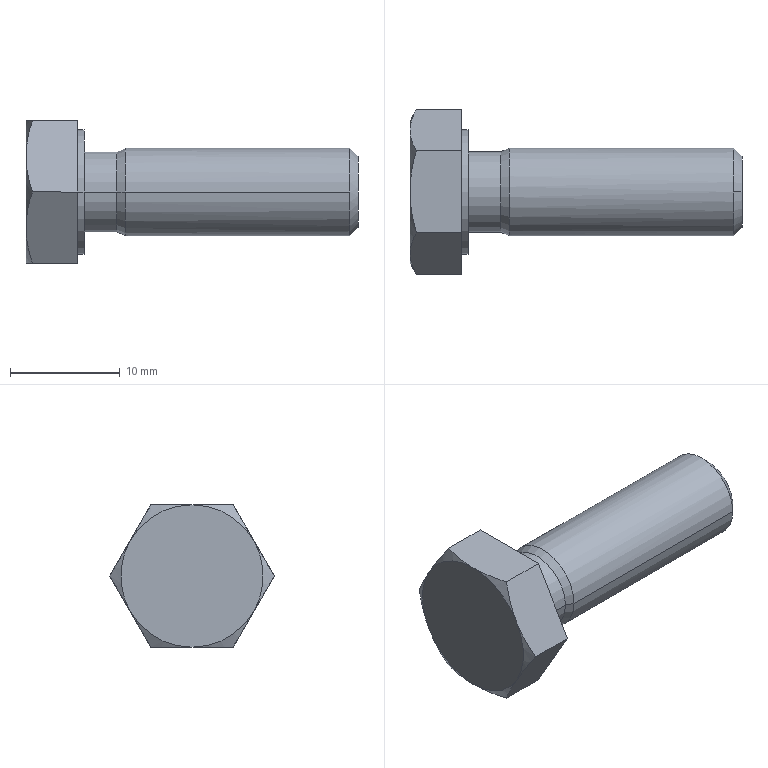Part | SolidWorks | features BaseBody 1 | 1 solid | 26 faces | box 30.3 x 15.011 x 13 mm | volume 1969 mm3 | cone 10 | plane 10 | cylinder 6 | commonest cylinder face diameters 7.323 x2 8 x2 11.4 x2
STEP:
#1=CARTESIAN_POINT('',(3.75,4.,0.));
#2=VERTEX_POINT('',#1);
#3=CARTESIAN_POINT('',(3.75,-4.,0.));
#4=VERTEX_POINT('',#3);
#5=CARTESIAN_POINT('',(3.75,0.,0.));
#6=DIRECTION('',(1.,0.,0.));
#7=DIRECTION('',(0.,1.,0.));
#8=AXIS2_PLACEMENT_3D('',#5,#6,#7);
#9=CIRCLE('',#8,4.);
#10=EDGE_CURVE('',#2,#4,#9,.T.);
#11=ORIENTED_EDGE('',*,*,#10,.T.);
#12=CARTESIAN_POINT('',(24.233,-4.,0.));
#13=VERTEX_POINT('',#12);
#14=CARTESIAN_POINT('',(14.375,-4.,0.));
#15=DIRECTION('',(1.,0.,0.));
#16=VECTOR('',#15,1000.);
#17=LINE('',#14,#16);
#18=EDGE_CURVE('',#4,#13,#17,.T.);
#19=ORIENTED_EDGE('',*,*,#18,.T.);
#20=CARTESIAN_POINT('',(24.233,0.,4.));
#21=VERTEX_POINT('',#20);
#22=CARTESIAN_POINT('',(24.233,0.,0.));
#23=DIRECTION('',(-1.,0.,0.));
#24=DIRECTION('',(0.,1.,0.));
#25=AXIS2_PLACEMENT_3D('',#22,#23,#24);
#26=CIRCLE('',#25,4.);
#27=EDGE_CURVE('',#13,#21,#26,.T.);
#28=ORIENTED_EDGE('',*,*,#27,.T.);
#29=CARTESIAN_POINT('',(24.233,4.,0.));
#30=VERTEX_POINT('',#29);
#31=CARTESIAN_POINT('',(24.233,0.,0.));
#32=DIRECTION('',(-1.,0.,0.));
#33=DIRECTION('',(0.,1.,0.));
#34=AXIS2_PLACEMENT_3D('',#31,#32,#33);
#35=CIRCLE('',#34,4.);
#36=EDGE_CURVE('',#21,#30,#35,.T.);
#37=ORIENTED_EDGE('',*,*,#36,.T.);
#38=CARTESIAN_POINT('',(14.375,4.,0.));
#39=DIRECTION('',(1.,0.,0.));
#40=VECTOR('',#39,1000.);
#41=LINE('',#38,#40);
#42=EDGE_CURVE('',#2,#30,#41,.T.);
#43=ORIENTED_EDGE('',*,*,#42,.F.);
#44=EDGE_LOOP('',(#11,#19,#28,#37,#43));
#45=FACE_OUTER_BOUND('',#44,.T.);
#46=CARTESIAN_POINT('',(14.375,0.,0.));
#47=DIRECTION('',(1.,0.,0.));
#48=DIRECTION('',(0.,1.,0.));
#49=AXIS2_PLACEMENT_3D('',#46,#47,#48);
#50=CYLINDRICAL_SURFACE('',#49,4.);
#51=ADVANCED_FACE('',(#45),#50,.T.);
#52=CARTESIAN_POINT('',(25.,0.,3.233));
#53=VERTEX_POINT('',#52);
#54=CARTESIAN_POINT('',(25.,0.,-3.233));
#55=VERTEX_POINT('',#54);
#56=CARTESIAN_POINT('',(25.,0.,0.));
#57=DIRECTION('',(-1.,0.,0.));
#58=DIRECTION('',(0.,0.,1.));
#59=AXIS2_PLACEMENT_3D('',#56,#57,#58);
#60=CIRCLE('',#59,3.233);
#61=EDGE_CURVE('',#53,#55,#60,.T.);
#62=ORIENTED_EDGE('',*,*,#61,.T.);
#63=CARTESIAN_POINT('',(24.233,0.,-4.));
#64=VERTEX_POINT('',#63);
#65=CARTESIAN_POINT('',(24.233,0.,-4.));
#66=DIRECTION('',(-0.7072,0.,-0.7071));
#67=VECTOR('',#66,1000.);
#68=LINE('',#65,#67);
#69=EDGE_CURVE('',#55,#64,#68,.T.);
#70=ORIENTED_EDGE('',*,*,#69,.T.);
#71=CARTESIAN_POINT('',(24.233,0.,0.));
#72=DIRECTION('',(-1.,0.,0.));
#73=DIRECTION('',(0.,1.,0.));
#74=AXIS2_PLACEMENT_3D('',#71,#72,#73);
#75=CIRCLE('',#74,4.);
#76=EDGE_CURVE('',#30,#64,#75,.T.);
#77=ORIENTED_EDGE('',*,*,#76,.F.);
#78=ORIENTED_EDGE('',*,*,#36,.F.);
#79=CARTESIAN_POINT('',(24.233,0.,4.));
#80=DIRECTION('',(-0.7072,0.,0.7071));
#81=VECTOR('',#80,1000.);
#82=LINE('',#79,#81);
#83=EDGE_CURVE('',#53,#21,#82,.T.);
#84=ORIENTED_EDGE('',*,*,#83,.F.);
#85=EDGE_LOOP('',(#62,#70,#77,#78,#84));
#86=FACE_OUTER_BOUND('',#85,.T.);
#87=CARTESIAN_POINT('',(24.233,0.,0.));
#88=DIRECTION('',(-1.,0.,0.));
#89=DIRECTION('',(0.,0.,1.));
#90=AXIS2_PLACEMENT_3D('',#87,#88,#89);
#91=CONICAL_SURFACE('',#90,4.,0.7853);
#92=ADVANCED_FACE('',(#86),#91,.T.);
#93=CARTESIAN_POINT('',(2.983,3.662,0.));
#94=VERTEX_POINT('',#93);
#95=CARTESIAN_POINT('',(2.983,-3.662,0.));
#96=VERTEX_POINT('',#95);
#97=CARTESIAN_POINT('',(2.983,0.,0.));
#98=DIRECTION('',(1.,0.,0.));
#99=DIRECTION('',(0.,1.,0.));
#100=AXIS2_PLACEMENT_3D('',#97,#98,#99);
#101=CIRCLE('',#100,3.662);
#102=EDGE_CURVE('',#94,#96,#101,.T.);
#103=ORIENTED_EDGE('',*,*,#102,.T.);
#104=CARTESIAN_POINT('',(3.75,-4.,0.));
#105=DIRECTION('',(0.9149,-0.4036,0.));
#106=VECTOR('',#105,1000.);
#107=LINE('',#104,#106);
#108=EDGE_CURVE('',#96,#4,#107,.T.);
#109=ORIENTED_EDGE('',*,*,#108,.T.);
#110=ORIENTED_EDGE('',*,*,#10,.F.);
#111=CARTESIAN_POINT('',(3.75,4.,0.));
#112=DIRECTION('',(0.9149,0.4036,0.));
#113=VECTOR('',#112,1000.);
#114=LINE('',#111,#113);
#115=EDGE_CURVE('',#94,#2,#114,.T.);
#116=ORIENTED_EDGE('',*,*,#115,.F.);
#117=EDGE_LOOP('',(#103,#109,#110,#116));
#118=FACE_OUTER_BOUND('',#117,.T.);
#119=CARTESIAN_POINT('',(3.75,0.,0.));
#120=DIRECTION('',(1.,0.,0.));
#121=DIRECTION('',(0.,1.,0.));
#122=AXIS2_PLACEMENT_3D('',#119,#120,#121);
#123=CONICAL_SURFACE('',#122,4.,0.4154);
#124=ADVANCED_FACE('',(#118),#123,.T.);
#125=CARTESIAN_POINT('',(0.,3.662,0.));
#126=VERTEX_POINT('',#125);
#127=CARTESIAN_POINT('',(0.,-3.662,0.));
#128=VERTEX_POINT('',#127);
#129=CARTESIAN_POINT('',(0.,0.,0.));
#130=DIRECTION('',(1.,0.,0.));
#131=DIRECTION('',(0.,1.,0.));
#132=AXIS2_PLACEMENT_3D('',#129,#130,#131);
#133=CIRCLE('',#132,3.662);
#134=EDGE_CURVE('',#126,#128,#133,.T.);
#135=ORIENTED_EDGE('',*,*,#134,.T.);
#136=CARTESIAN_POINT('',(1.492,-3.662,0.));
#137=DIRECTION('',(1.,0.,0.));
#138=VECTOR('',#137,1000.);
#139=LINE('',#136,#138);
#140=EDGE_CURVE('',#128,#96,#139,.T.);
#141=ORIENTED_EDGE('',*,*,#140,.T.);
#142=ORIENTED_EDGE('',*,*,#102,.F.);
#143=CARTESIAN_POINT('',(1.492,3.662,0.));
#144=DIRECTION('',(1.,0.,0.));
#145=VECTOR('',#144,1000.);
#146=LINE('',#143,#145);
#147=EDGE_CURVE('',#126,#94,#146,.T.);
#148=ORIENTED_EDGE('',*,*,#147,.F.);
#149=EDGE_LOOP('',(#135,#141,#142,#148));
#150=FACE_OUTER_BOUND('',#149,.T.);
#151=CARTESIAN_POINT('',(1.492,0.,0.));
#152=DIRECTION('',(1.,0.,0.));
#153=DIRECTION('',(0.,1.,0.));
#154=AXIS2_PLACEMENT_3D('',#151,#152,#153);
#155=CYLINDRICAL_SURFACE('',#154,3.662);
#156=ADVANCED_FACE('',(#150),#155,.T.);
#157=CARTESIAN_POINT('',(-0.6001,5.7,0.));
#158=VERTEX_POINT('',#157);
#159=CARTESIAN_POINT('',(-0.6001,-5.7,0.));
#160=VERTEX_POINT('',#159);
#161=CARTESIAN_POINT('',(-0.6001,0.,0.));
#162=DIRECTION('',(1.,0.,0.));
#163=DIRECTION('',(0.,1.,0.));
#164=AXIS2_PLACEMENT_3D('',#161,#162,#163);
#165=CIRCLE('',#164,5.7);
#166=EDGE_CURVE('',#158,#160,#165,.T.);
#167=ORIENTED_EDGE('',*,*,#166,.T.);
#168=CARTESIAN_POINT('',(0.,-5.7,0.));
#169=VERTEX_POINT('',#168);
#170=CARTESIAN_POINT('',(-0.3,-5.7,0.));
#171=DIRECTION('',(1.,0.,0.));
#172=VECTOR('',#171,1000.);
#173=LINE('',#170,#172);
#174=EDGE_CURVE('',#160,#169,#173,.T.);
#175=ORIENTED_EDGE('',*,*,#174,.T.);
#176=CARTESIAN_POINT('',(0.,5.7,0.));
#177=VERTEX_POINT('',#176);
#178=CARTESIAN_POINT('',(0.,0.,0.));
#179=DIRECTION('',(1.,0.,0.));
#180=DIRECTION('',(0.,1.,0.));
#181=AXIS2_PLACEMENT_3D('',#178,#179,#180);
#182=CIRCLE('',#181,5.7);
#183=EDGE_CURVE('',#177,#169,#182,.T.);
#184=ORIENTED_EDGE('',*,*,#183,.F.);
#185=CARTESIAN_POINT('',(-0.3,5.7,0.));
#186=DIRECTION('',(1.,0.,0.));
#187=VECTOR('',#186,1000.);
#188=LINE('',#185,#187);
#189=EDGE_CURVE('',#158,#177,#188,.T.);
#190=ORIENTED_EDGE('',*,*,#189,.F.);
#191=EDGE_LOOP('',(#167,#175,#184,#190));
#192=FACE_OUTER_BOUND('',#191,.T.);
#193=CARTESIAN_POINT('',(-0.3,0.,0.));
#194=DIRECTION('',(1.,0.,0.));
#195=DIRECTION('',(0.,1.,0.));
#196=AXIS2_PLACEMENT_3D('',#193,#194,#195);
#197=CYLINDRICAL_SURFACE('',#196,5.7);
#198=ADVANCED_FACE('',(#192),#197,.T.);
#199=ORIENTED_EDGE('',*,*,#18,.F.);
#200=CARTESIAN_POINT('',(3.75,0.,0.));
#201=DIRECTION('',(1.,0.,0.));
#202=DIRECTION('',(0.,1.,0.));
#203=AXIS2_PLACEMENT_3D('',#200,#201,#202);
#204=CIRCLE('',#203,4.);
#205=EDGE_CURVE('',#4,#2,#204,.T.);
#206=ORIENTED_EDGE('',*,*,#205,.T.);
#207=ORIENTED_EDGE('',*,*,#42,.T.);
#208=ORIENTED_EDGE('',*,*,#76,.T.);
#209=CARTESIAN_POINT('',(24.233,0.,0.));
#210=DIRECTION('',(-1.,0.,0.));
#211=DIRECTION('',(0.,1.,0.));
#212=AXIS2_PLACEMENT_3D('',#209,#210,#211);
#213=CIRCLE('',#212,4.);
#214=EDGE_CURVE('',#64,#13,#213,.T.);
#215=ORIENTED_EDGE('',*,*,#214,.T.);
#216=EDGE_LOOP('',(#199,#206,#207,#208,#215));
#217=FACE_OUTER_BOUND('',#216,.T.);
#218=CARTESIAN_POINT('',(14.375,0.,0.));
#219=DIRECTION('',(1.,0.,0.));
#220=DIRECTION('',(0.,1.,0.));
#221=AXIS2_PLACEMENT_3D('',#218,#219,#220);
#222=CYLINDRICAL_SURFACE('',#221,4.);
#223=ADVANCED_FACE('',(#217),#222,.T.);
#224=ORIENTED_EDGE('',*,*,#69,.F.);
#225=CARTESIAN_POINT('',(25.,0.,0.));
#226=DIRECTION('',(-1.,0.,0.));
#227=DIRECTION('',(0.,0.,1.));
#228=AXIS2_PLACEMENT_3D('',#225,#226,#227);
#229=CIRCLE('',#228,3.233);
#230=EDGE_CURVE('',#55,#53,#229,.T.);
#231=ORIENTED_EDGE('',*,*,#230,.T.);
#232=ORIENTED_EDGE('',*,*,#83,.T.);
#233=ORIENTED_EDGE('',*,*,#27,.F.);
#234=ORIENTED_EDGE('',*,*,#214,.F.);
#235=EDGE_LOOP('',(#224,#231,#232,#233,#234));
#236=FACE_OUTER_BOUND('',#235,.T.);
#237=CARTESIAN_POINT('',(24.233,0.,0.));
#238=DIRECTION('',(-1.,0.,0.));
#239=DIRECTION('',(0.,0.,1.));
#240=AXIS2_PLACEMENT_3D('',#237,#238,#239);
#241=CONICAL_SURFACE('',#240,4.,0.7853);
#242=ADVANCED_FACE('',(#236),#241,.T.);
#243=ORIENTED_EDGE('',*,*,#108,.F.);
#244=CARTESIAN_POINT('',(2.983,0.,0.));
#245=DIRECTION('',(1.,0.,0.));
#246=DIRECTION('',(0.,1.,0.));
#247=AXIS2_PLACEMENT_3D('',#244,#245,#246);
#248=CIRCLE('',#247,3.662);
#249=EDGE_CURVE('',#96,#94,#248,.T.);
#250=ORIENTED_EDGE('',*,*,#249,.T.);
#251=ORIENTED_EDGE('',*,*,#115,.T.);
#252=ORIENTED_EDGE('',*,*,#205,.F.);
#253=EDGE_LOOP('',(#243,#250,#251,#252));
#254=FACE_OUTER_BOUND('',#253,.T.);
#255=CARTESIAN_POINT('',(3.75,0.,0.));
#256=DIRECTION('',(1.,0.,0.));
#257=DIRECTION('',(0.,1.,0.));
#258=AXIS2_PLACEMENT_3D('',#255,#256,#257);
#259=CONICAL_SURFACE('',#258,4.,0.4154);
#260=ADVANCED_FACE('',(#254),#259,.T.);
#261=ORIENTED_EDGE('',*,*,#61,.F.);
#262=ORIENTED_EDGE('',*,*,#230,.F.);
#263=EDGE_LOOP('',(#261,#262));
#264=FACE_OUTER_BOUND('',#263,.T.);
#265=CARTESIAN_POINT('',(25.,2.,0.));
#266=DIRECTION('',(1.,0.,0.));
#267=DIRECTION('',(0.,1.,0.));
#268=AXIS2_PLACEMENT_3D('',#265,#266,#267);
#269=PLANE('',#268);
#270=ADVANCED_FACE('',(#264),#269,.T.);
#271=ORIENTED_EDGE('',*,*,#140,.F.);
#272=CARTESIAN_POINT('',(0.,0.,0.));
#273=DIRECTION('',(1.,0.,0.));
#274=DIRECTION('',(0.,1.,0.));
#275=AXIS2_PLACEMENT_3D('',#272,#273,#274);
#276=CIRCLE('',#275,3.662);
#277=EDGE_CURVE('',#128,#126,#276,.T.);
#278=ORIENTED_EDGE('',*,*,#277,.T.);
#279=ORIENTED_EDGE('',*,*,#147,.T.);
#280=ORIENTED_EDGE('',*,*,#249,.F.);
#281=EDGE_LOOP('',(#271,#278,#279,#280));
#282=FACE_OUTER_BOUND('',#281,.T.);
#283=CARTESIAN_POINT('',(1.492,0.,0.));
#284=DIRECTION('',(1.,0.,0.));
#285=DIRECTION('',(0.,1.,0.));
#286=AXIS2_PLACEMENT_3D('',#283,#284,#285);
#287=CYLINDRICAL_SURFACE('',#286,3.662);
#288=ADVANCED_FACE('',(#282),#287,.T.);
#289=ORIENTED_EDGE('',*,*,#134,.F.);
#290=ORIENTED_EDGE('',*,*,#277,.F.);
#291=EDGE_LOOP('',(#289,#290));
#292=FACE_BOUND('',#291,.T.);
#293=ORIENTED_EDGE('',*,*,#183,.T.);
#294=CARTESIAN_POINT('',(0.,0.,0.));
#295=DIRECTION('',(1.,0.,0.));
#296=DIRECTION('',(0.,1.,0.));
#297=AXIS2_PLACEMENT_3D('',#294,#295,#296);
#298=CIRCLE('',#297,5.7);
#299=EDGE_CURVE('',#169,#177,#298,.T.);
#300=ORIENTED_EDGE('',*,*,#299,.T.);
#301=EDGE_LOOP('',(#293,#300));
#302=FACE_OUTER_BOUND('',#301,.T.);
#303=CARTESIAN_POINT('',(0.,4.681,0.));
#304=DIRECTION('',(1.,0.,0.));
#305=DIRECTION('',(0.,1.,0.));
#306=AXIS2_PLACEMENT_3D('',#303,#304,#305);
#307=PLANE('',#306);
#308=ADVANCED_FACE('',(#292,#302),#307,.T.);
#309=ORIENTED_EDGE('',*,*,#174,.F.);
#310=CARTESIAN_POINT('',(-0.6001,0.,0.));
#311=DIRECTION('',(1.,0.,0.));
#312=DIRECTION('',(0.,1.,0.));
#313=AXIS2_PLACEMENT_3D('',#310,#311,#312);
#314=CIRCLE('',#313,5.7);
#315=EDGE_CURVE('',#160,#158,#314,.T.);
#316=ORIENTED_EDGE('',*,*,#315,.T.);
#317=ORIENTED_EDGE('',*,*,#189,.T.);
#318=ORIENTED_EDGE('',*,*,#299,.F.);
#319=EDGE_LOOP('',(#309,#316,#317,#318));
#320=FACE_OUTER_BOUND('',#319,.T.);
#321=CARTESIAN_POINT('',(-0.3,0.,0.));
#322=DIRECTION('',(1.,0.,0.));
#323=DIRECTION('',(0.,1.,0.));
#324=AXIS2_PLACEMENT_3D('',#321,#322,#323);
#325=CYLINDRICAL_SURFACE('',#324,5.7);
#326=ADVANCED_FACE('',(#320),#325,.T.);
#327=ORIENTED_EDGE('',*,*,#166,.F.);
#328=ORIENTED_EDGE('',*,*,#315,.F.);
#329=EDGE_LOOP('',(#327,#328));
#330=FACE_BOUND('',#329,.T.);
#331=CARTESIAN_POINT('',(-0.6001,-3.753,-6.5));
#332=VERTEX_POINT('',#331);
#333=CARTESIAN_POINT('',(-0.6001,3.753,-6.5));
#334=VERTEX_POINT('',#333);
#335=CARTESIAN_POINT('',(-0.6001,0.,-6.5));
#336=DIRECTION('',(0.,1.,0.));
#337=VECTOR('',#336,1000.);
#338=LINE('',#335,#337);
#339=EDGE_CURVE('',#332,#334,#338,.T.);
#340=ORIENTED_EDGE('',*,*,#339,.T.);
#341=CARTESIAN_POINT('',(-0.6001,7.506,0.));
#342=VERTEX_POINT('',#341);
#343=CARTESIAN_POINT('',(-0.6001,3.753,-6.5));
#344=DIRECTION('',(0.,0.5,0.866));
#345=VECTOR('',#344,1000.);
#346=LINE('',#343,#345);
#347=EDGE_CURVE('',#334,#342,#346,.T.);
#348=ORIENTED_EDGE('',*,*,#347,.T.);
#349=CARTESIAN_POINT('',(-0.6001,3.753,6.5));
#350=VERTEX_POINT('',#349);
#351=CARTESIAN_POINT('',(-0.6001,7.506,0.));
#352=DIRECTION('',(0.,-0.5,0.866));
#353=VECTOR('',#352,1000.);
#354=LINE('',#351,#353);
#355=EDGE_CURVE('',#342,#350,#354,.T.);
#356=ORIENTED_EDGE('',*,*,#355,.T.);
#357=CARTESIAN_POINT('',(-0.6001,-3.753,6.5));
#358=VERTEX_POINT('',#357);
#359=CARTESIAN_POINT('',(-0.6001,0.,6.5));
#360=DIRECTION('',(0.,-1.,0.));
#361=VECTOR('',#360,1000.);
#362=LINE('',#359,#361);
#363=EDGE_CURVE('',#350,#358,#362,.T.);
#364=ORIENTED_EDGE('',*,*,#363,.T.);
#365=CARTESIAN_POINT('',(-0.6001,-7.506,0.));
#366=VERTEX_POINT('',#365);
#367=CARTESIAN_POINT('',(-0.6001,-3.753,6.5));
#368=DIRECTION('',(0.,-0.5,-0.866));
#369=VECTOR('',#368,1000.);
#370=LINE('',#367,#369);
#371=EDGE_CURVE('',#358,#366,#370,.T.);
#372=ORIENTED_EDGE('',*,*,#371,.T.);
#373=CARTESIAN_POINT('',(-0.6001,-7.506,0.));
#374=DIRECTION('',(0.,0.5,-0.866));
#375=VECTOR('',#374,1000.);
#376=LINE('',#373,#375);
#377=EDGE_CURVE('',#366,#332,#376,.T.);
#378=ORIENTED_EDGE('',*,*,#377,.T.);
#379=EDGE_LOOP('',(#340,#348,#356,#364,#372,#378));
#380=FACE_OUTER_BOUND('',#379,.T.);
#381=CARTESIAN_POINT('',(-0.6001,0.,0.));
#382=DIRECTION('',(1.,0.,0.));
#383=DIRECTION('',(0.,1.,0.));
#384=AXIS2_PLACEMENT_3D('',#381,#382,#383);
#385=PLANE('',#384);
#386=ADVANCED_FACE('',(#330,#380),#385,.T.);
#387=ORIENTED_EDGE('',*,*,#347,.F.);
#388=CARTESIAN_POINT('',(-4.72,3.753,-6.5));
#389=VERTEX_POINT('',#388);
#390=CARTESIAN_POINT('',(-0.6001,3.753,-6.5));
#391=DIRECTION('',(-1.,0.,0.));
#392=VECTOR('',#391,1000.);
#393=LINE('',#390,#392);
#394=EDGE_CURVE('',#334,#389,#393,.T.);
#395=ORIENTED_EDGE('',*,*,#394,.T.);
#396=CARTESIAN_POINT('',(-5.3,5.629,-3.25));
#397=VERTEX_POINT('',#396);
#398=CARTESIAN_POINT('',(-4.72,3.753,-6.5));
#399=CARTESIAN_POINT('',(-5.073,4.366,-5.438));
#400=CARTESIAN_POINT('',(-5.3,4.989,-4.359));
#401=CARTESIAN_POINT('',(-5.3,5.629,-3.25));
#402=B_SPLINE_CURVE_WITH_KNOTS('',3,(#398,#399,#400,#401),.UNSPECIFIED.,.F.,.F.,(4,4),(0.,0.003797),.UNSPECIFIED.);
#403=EDGE_CURVE('',#389,#397,#402,.T.);
#404=ORIENTED_EDGE('',*,*,#403,.T.);
#405=CARTESIAN_POINT('',(-4.72,7.506,0.));
#406=VERTEX_POINT('',#405);
#407=CARTESIAN_POINT('',(-5.3,5.629,-3.25));
#408=CARTESIAN_POINT('',(-5.3,6.27,-2.141));
#409=CARTESIAN_POINT('',(-5.073,6.892,-1.062));
#410=CARTESIAN_POINT('',(-4.72,7.506,0.));
#411=B_SPLINE_CURVE_WITH_KNOTS('',3,(#407,#408,#409,#410),.UNSPECIFIED.,.F.,.F.,(4,4),(0.,0.003797),.UNSPECIFIED.);
#412=EDGE_CURVE('',#397,#406,#411,.T.);
#413=ORIENTED_EDGE('',*,*,#412,.T.);
#414=CARTESIAN_POINT('',(-0.6001,7.506,0.));
#415=DIRECTION('',(1.,0.,0.));
#416=VECTOR('',#415,1000.);
#417=LINE('',#414,#416);
#418=EDGE_CURVE('',#406,#342,#417,.T.);
#419=ORIENTED_EDGE('',*,*,#418,.T.);
#420=EDGE_LOOP('',(#387,#395,#404,#413,#419));
#421=FACE_OUTER_BOUND('',#420,.T.);
#422=CARTESIAN_POINT('',(-0.6001,3.753,-6.5));
#423=DIRECTION('',(0.,0.866,-0.5));
#424=DIRECTION('',(0.,0.5,0.866));
#425=AXIS2_PLACEMENT_3D('',#422,#423,#424);
#426=PLANE('',#425);
#427=ADVANCED_FACE('',(#421),#426,.T.);
#428=ORIENTED_EDGE('',*,*,#339,.F.);
#429=CARTESIAN_POINT('',(-4.72,-3.753,-6.5));
#430=VERTEX_POINT('',#429);
#431=CARTESIAN_POINT('',(-0.6001,-3.753,-6.5));
#432=DIRECTION('',(-1.,0.,0.));
#433=VECTOR('',#432,1000.);
#434=LINE('',#431,#433);
#435=EDGE_CURVE('',#332,#430,#434,.T.);
#436=ORIENTED_EDGE('',*,*,#435,.T.);
#437=CARTESIAN_POINT('',(-5.3,0.,-6.5));
#438=VERTEX_POINT('',#437);
#439=CARTESIAN_POINT('',(-4.72,-3.753,-6.5));
#440=CARTESIAN_POINT('',(-5.073,-2.527,-6.5));
#441=CARTESIAN_POINT('',(-5.3,-1.281,-6.5));
#442=CARTESIAN_POINT('',(-5.3,0.,-6.5));
#443=B_SPLINE_CURVE_WITH_KNOTS('',3,(#439,#440,#441,#442),.UNSPECIFIED.,.F.,.F.,(4,4),(0.,0.003797),.UNSPECIFIED.);
#444=EDGE_CURVE('',#430,#438,#443,.T.);
#445=ORIENTED_EDGE('',*,*,#444,.T.);
#446=CARTESIAN_POINT('',(-5.3,0.,-6.5));
#447=CARTESIAN_POINT('',(-5.3,1.281,-6.5));
#448=CARTESIAN_POINT('',(-5.073,2.527,-6.5));
#449=CARTESIAN_POINT('',(-4.72,3.753,-6.5));
#450=B_SPLINE_CURVE_WITH_KNOTS('',3,(#446,#447,#448,#449),.UNSPECIFIED.,.F.,.F.,(4,4),(0.,0.003797),.UNSPECIFIED.);
#451=EDGE_CURVE('',#438,#389,#450,.T.);
#452=ORIENTED_EDGE('',*,*,#451,.T.);
#453=ORIENTED_EDGE('',*,*,#394,.F.);
#454=EDGE_LOOP('',(#428,#436,#445,#452,#453));
#455=FACE_OUTER_BOUND('',#454,.T.);
#456=CARTESIAN_POINT('',(-0.6001,-3.753,-6.5));
#457=DIRECTION('',(0.,0.,-1.));
#458=DIRECTION('',(0.,1.,0.));
#459=AXIS2_PLACEMENT_3D('',#456,#457,#458);
#460=PLANE('',#459);
#461=ADVANCED_FACE('',(#455),#460,.T.);
#462=CARTESIAN_POINT('',(-4.72,-7.506,0.));
#463=VERTEX_POINT('',#462);
#464=CARTESIAN_POINT('',(-0.6001,-7.506,0.));
#465=DIRECTION('',(-1.,0.,0.));
#466=VECTOR('',#465,1000.);
#467=LINE('',#464,#466);
#468=EDGE_CURVE('',#366,#463,#467,.T.);
#469=ORIENTED_EDGE('',*,*,#468,.T.);
#470=CARTESIAN_POINT('',(-5.3,-5.629,-3.25));
#471=VERTEX_POINT('',#470);
#472=CARTESIAN_POINT('',(-4.72,-7.506,0.));
#473=CARTESIAN_POINT('',(-5.073,-6.892,-1.062));
#474=CARTESIAN_POINT('',(-5.3,-6.27,-2.141));
#475=CARTESIAN_POINT('',(-5.3,-5.629,-3.25));
#476=B_SPLINE_CURVE_WITH_KNOTS('',3,(#472,#473,#474,#475),.UNSPECIFIED.,.F.,.F.,(4,4),(0.,0.003797),.UNSPECIFIED.);
#477=EDGE_CURVE('',#463,#471,#476,.T.);
#478=ORIENTED_EDGE('',*,*,#477,.T.);
#479=CARTESIAN_POINT('',(-5.3,-5.629,-3.25));
#480=CARTESIAN_POINT('',(-5.3,-4.989,-4.359));
#481=CARTESIAN_POINT('',(-5.073,-4.366,-5.438));
#482=CARTESIAN_POINT('',(-4.72,-3.753,-6.5));
#483=B_SPLINE_CURVE_WITH_KNOTS('',3,(#479,#480,#481,#482),.UNSPECIFIED.,.F.,.F.,(4,4),(0.,0.003797),.UNSPECIFIED.);
#484=EDGE_CURVE('',#471,#430,#483,.T.);
#485=ORIENTED_EDGE('',*,*,#484,.T.);
#486=ORIENTED_EDGE('',*,*,#435,.F.);
#487=ORIENTED_EDGE('',*,*,#377,.F.);
#488=EDGE_LOOP('',(#469,#478,#485,#486,#487));
#489=FACE_OUTER_BOUND('',#488,.T.);
#490=CARTESIAN_POINT('',(-0.6001,-7.506,0.));
#491=DIRECTION('',(0.,-0.866,-0.5));
#492=DIRECTION('',(0.,0.5,-0.866));
#493=AXIS2_PLACEMENT_3D('',#490,#491,#492);
#494=PLANE('',#493);
#495=ADVANCED_FACE('',(#489),#494,.T.);
#496=CARTESIAN_POINT('',(-4.72,-3.753,6.5));
#497=VERTEX_POINT('',#496);
#498=CARTESIAN_POINT('',(-0.6001,-3.753,6.5));
#499=DIRECTION('',(-1.,0.,0.));
#500=VECTOR('',#499,1000.);
#501=LINE('',#498,#500);
#502=EDGE_CURVE('',#358,#497,#501,.T.);
#503=ORIENTED_EDGE('',*,*,#502,.T.);
#504=CARTESIAN_POINT('',(-5.3,-5.629,3.25));
#505=VERTEX_POINT('',#504);
#506=CARTESIAN_POINT('',(-4.72,-3.753,6.5));
#507=CARTESIAN_POINT('',(-5.073,-4.366,5.438));
#508=CARTESIAN_POINT('',(-5.3,-4.989,4.359));
#509=CARTESIAN_POINT('',(-5.3,-5.629,3.25));
#510=B_SPLINE_CURVE_WITH_KNOTS('',3,(#506,#507,#508,#509),.UNSPECIFIED.,.F.,.F.,(4,4),(0.,0.003797),.UNSPECIFIED.);
#511=EDGE_CURVE('',#497,#505,#510,.T.);
#512=ORIENTED_EDGE('',*,*,#511,.T.);
#513=CARTESIAN_POINT('',(-5.3,-5.629,3.25));
#514=CARTESIAN_POINT('',(-5.3,-6.27,2.141));
#515=CARTESIAN_POINT('',(-5.073,-6.892,1.062));
#516=CARTESIAN_POINT('',(-4.72,-7.506,0.));
#517=B_SPLINE_CURVE_WITH_KNOTS('',3,(#513,#514,#515,#516),.UNSPECIFIED.,.F.,.F.,(4,4),(0.,0.003797),.UNSPECIFIED.);
#518=EDGE_CURVE('',#505,#463,#517,.T.);
#519=ORIENTED_EDGE('',*,*,#518,.T.);
#520=ORIENTED_EDGE('',*,*,#468,.F.);
#521=ORIENTED_EDGE('',*,*,#371,.F.);
#522=EDGE_LOOP('',(#503,#512,#519,#520,#521));
#523=FACE_OUTER_BOUND('',#522,.T.);
#524=CARTESIAN_POINT('',(-0.6001,-3.753,6.5));
#525=DIRECTION('',(0.,-0.866,0.5));
#526=DIRECTION('',(0.,-0.5,-0.866));
#527=AXIS2_PLACEMENT_3D('',#524,#525,#526);
#528=PLANE('',#527);
#529=ADVANCED_FACE('',(#523),#528,.T.);
#530=CARTESIAN_POINT('',(-4.72,3.753,6.5));
#531=VERTEX_POINT('',#530);
#532=CARTESIAN_POINT('',(-0.6001,3.753,6.5));
#533=DIRECTION('',(-1.,0.,0.));
#534=VECTOR('',#533,1000.);
#535=LINE('',#532,#534);
#536=EDGE_CURVE('',#350,#531,#535,.T.);
#537=ORIENTED_EDGE('',*,*,#536,.T.);
#538=CARTESIAN_POINT('',(-5.3,0.,6.5));
#539=VERTEX_POINT('',#538);
#540=CARTESIAN_POINT('',(-4.72,3.753,6.5));
#541=CARTESIAN_POINT('',(-5.073,2.527,6.5));
#542=CARTESIAN_POINT('',(-5.3,1.281,6.5));
#543=CARTESIAN_POINT('',(-5.3,0.,6.5));
#544=B_SPLINE_CURVE_WITH_KNOTS('',3,(#540,#541,#542,#543),.UNSPECIFIED.,.F.,.F.,(4,4),(0.,0.003797),.UNSPECIFIED.);
#545=EDGE_CURVE('',#531,#539,#544,.T.);
#546=ORIENTED_EDGE('',*,*,#545,.T.);
#547=CARTESIAN_POINT('',(-5.3,0.,6.5));
#548=CARTESIAN_POINT('',(-5.3,-1.281,6.5));
#549=CARTESIAN_POINT('',(-5.073,-2.527,6.5));
#550=CARTESIAN_POINT('',(-4.72,-3.753,6.5));
#551=B_SPLINE_CURVE_WITH_KNOTS('',3,(#547,#548,#549,#550),.UNSPECIFIED.,.F.,.F.,(4,4),(0.,0.003797),.UNSPECIFIED.);
#552=EDGE_CURVE('',#539,#497,#551,.T.);
#553=ORIENTED_EDGE('',*,*,#552,.T.);
#554=ORIENTED_EDGE('',*,*,#502,.F.);
#555=ORIENTED_EDGE('',*,*,#363,.F.);
#556=EDGE_LOOP('',(#537,#546,#553,#554,#555));
#557=FACE_OUTER_BOUND('',#556,.T.);
#558=CARTESIAN_POINT('',(-0.6001,3.753,6.5));
#559=DIRECTION('',(0.,0.,1.));
#560=DIRECTION('',(0.,-1.,0.));
#561=AXIS2_PLACEMENT_3D('',#558,#559,#560);
#562=PLANE('',#561);
#563=ADVANCED_FACE('',(#557),#562,.T.);
#564=ORIENTED_EDGE('',*,*,#355,.F.);
#565=ORIENTED_EDGE('',*,*,#418,.F.);
#566=CARTESIAN_POINT('',(-5.3,5.629,3.25));
#567=VERTEX_POINT('',#566);
#568=CARTESIAN_POINT('',(-4.72,7.506,0.));
#569=CARTESIAN_POINT('',(-5.073,6.892,1.062));
#570=CARTESIAN_POINT('',(-5.3,6.27,2.141));
#571=CARTESIAN_POINT('',(-5.3,5.629,3.25));
#572=B_SPLINE_CURVE_WITH_KNOTS('',3,(#568,#569,#570,#571),.UNSPECIFIED.,.F.,.F.,(4,4),(0.,0.003797),.UNSPECIFIED.);
#573=EDGE_CURVE('',#406,#567,#572,.T.);
#574=ORIENTED_EDGE('',*,*,#573,.T.);
#575=CARTESIAN_POINT('',(-5.3,5.629,3.25));
#576=CARTESIAN_POINT('',(-5.3,4.989,4.359));
#577=CARTESIAN_POINT('',(-5.073,4.366,5.438));
#578=CARTESIAN_POINT('',(-4.72,3.753,6.5));
#579=B_SPLINE_CURVE_WITH_KNOTS('',3,(#575,#576,#577,#578),.UNSPECIFIED.,.F.,.F.,(4,4),(0.,0.003797),.UNSPECIFIED.);
#580=EDGE_CURVE('',#567,#531,#579,.T.);
#581=ORIENTED_EDGE('',*,*,#580,.T.);
#582=ORIENTED_EDGE('',*,*,#536,.F.);
#583=EDGE_LOOP('',(#564,#565,#574,#581,#582));
#584=FACE_OUTER_BOUND('',#583,.T.);
#585=CARTESIAN_POINT('',(-0.6001,7.506,0.));
#586=DIRECTION('',(0.,0.866,0.5));
#587=DIRECTION('',(0.,-0.5,0.866));
#588=AXIS2_PLACEMENT_3D('',#585,#586,#587);
#589=PLANE('',#588);
#590=ADVANCED_FACE('',(#584),#589,.T.);
#591=CARTESIAN_POINT('',(-5.3,0.,0.));
#592=DIRECTION('',(1.,0.,0.));
#593=DIRECTION('',(0.,0.,-1.));
#594=AXIS2_PLACEMENT_3D('',#591,#592,#593);
#595=CIRCLE('',#594,6.5);
#596=EDGE_CURVE('',#397,#567,#595,.T.);
#597=ORIENTED_EDGE('',*,*,#596,.T.);
#598=ORIENTED_EDGE('',*,*,#573,.F.);
#599=ORIENTED_EDGE('',*,*,#412,.F.);
#600=EDGE_LOOP('',(#597,#598,#599));
#601=FACE_OUTER_BOUND('',#600,.T.);
#602=CARTESIAN_POINT('',(-4.716,0.,0.));
#603=DIRECTION('',(1.,0.,0.));
#604=DIRECTION('',(0.,0.,-1.));
#605=AXIS2_PLACEMENT_3D('',#602,#603,#604);
#606=CONICAL_SURFACE('',#605,7.512,1.047);
#607=ADVANCED_FACE('',(#601),#606,.T.);
#608=CARTESIAN_POINT('',(-5.3,0.,0.));
#609=DIRECTION('',(1.,0.,0.));
#610=DIRECTION('',(0.,0.,-1.));
#611=AXIS2_PLACEMENT_3D('',#608,#609,#610);
#612=CIRCLE('',#611,6.5);
#613=EDGE_CURVE('',#438,#397,#612,.T.);
#614=ORIENTED_EDGE('',*,*,#613,.T.);
#615=ORIENTED_EDGE('',*,*,#403,.F.);
#616=ORIENTED_EDGE('',*,*,#451,.F.);
#617=EDGE_LOOP('',(#614,#615,#616));
#618=FACE_OUTER_BOUND('',#617,.T.);
#619=CARTESIAN_POINT('',(-4.716,0.,0.));
#620=DIRECTION('',(1.,0.,0.));
#621=DIRECTION('',(0.,0.,-1.));
#622=AXIS2_PLACEMENT_3D('',#619,#620,#621);
#623=CONICAL_SURFACE('',#622,7.512,1.047);
#624=ADVANCED_FACE('',(#618),#623,.T.);
#625=ORIENTED_EDGE('',*,*,#484,.F.);
#626=CARTESIAN_POINT('',(-5.3,0.,0.));
#627=DIRECTION('',(1.,0.,0.));
#628=DIRECTION('',(0.,0.,-1.));
#629=AXIS2_PLACEMENT_3D('',#626,#627,#628);
#630=CIRCLE('',#629,6.5);
#631=EDGE_CURVE('',#471,#438,#630,.T.);
#632=ORIENTED_EDGE('',*,*,#631,.T.);
#633=ORIENTED_EDGE('',*,*,#444,.F.);
#634=EDGE_LOOP('',(#625,#632,#633));
#635=FACE_OUTER_BOUND('',#634,.T.);
#636=CARTESIAN_POINT('',(-4.716,0.,0.));
#637=DIRECTION('',(1.,0.,0.));
#638=DIRECTION('',(0.,0.,-1.));
#639=AXIS2_PLACEMENT_3D('',#636,#637,#638);
#640=CONICAL_SURFACE('',#639,7.512,1.047);
#641=ADVANCED_FACE('',(#635),#640,.T.);
#642=ORIENTED_EDGE('',*,*,#518,.F.);
#643=CARTESIAN_POINT('',(-5.3,0.,0.));
#644=DIRECTION('',(1.,0.,0.));
#645=DIRECTION('',(0.,0.,-1.));
#646=AXIS2_PLACEMENT_3D('',#643,#644,#645);
#647=CIRCLE('',#646,6.5);
#648=EDGE_CURVE('',#505,#471,#647,.T.);
#649=ORIENTED_EDGE('',*,*,#648,.T.);
#650=ORIENTED_EDGE('',*,*,#477,.F.);
#651=EDGE_LOOP('',(#642,#649,#650));
#652=FACE_OUTER_BOUND('',#651,.T.);
#653=CARTESIAN_POINT('',(-4.716,0.,0.));
#654=DIRECTION('',(1.,0.,0.));
#655=DIRECTION('',(0.,0.,-1.));
#656=AXIS2_PLACEMENT_3D('',#653,#654,#655);
#657=CONICAL_SURFACE('',#656,7.512,1.047);
#658=ADVANCED_FACE('',(#652),#657,.T.);
#659=ORIENTED_EDGE('',*,*,#552,.F.);
#660=CARTESIAN_POINT('',(-5.3,0.,0.));
#661=DIRECTION('',(1.,0.,0.));
#662=DIRECTION('',(0.,0.,-1.));
#663=AXIS2_PLACEMENT_3D('',#660,#661,#662);
#664=CIRCLE('',#663,6.5);
#665=EDGE_CURVE('',#539,#505,#664,.T.);
#666=ORIENTED_EDGE('',*,*,#665,.T.);
#667=ORIENTED_EDGE('',*,*,#511,.F.);
#668=EDGE_LOOP('',(#659,#666,#667));
#669=FACE_OUTER_BOUND('',#668,.T.);
#670=CARTESIAN_POINT('',(-4.716,0.,0.));
#671=DIRECTION('',(1.,0.,0.));
#672=DIRECTION('',(0.,0.,-1.));
#673=AXIS2_PLACEMENT_3D('',#670,#671,#672);
#674=CONICAL_SURFACE('',#673,7.512,1.047);
#675=ADVANCED_FACE('',(#669),#674,.T.);
#676=CARTESIAN_POINT('',(-5.3,0.,0.));
#677=DIRECTION('',(1.,0.,0.));
#678=DIRECTION('',(0.,0.,-1.));
#679=AXIS2_PLACEMENT_3D('',#676,#677,#678);
#680=CIRCLE('',#679,6.5);
#681=EDGE_CURVE('',#567,#539,#680,.T.);
#682=ORIENTED_EDGE('',*,*,#681,.T.);
#683=ORIENTED_EDGE('',*,*,#545,.F.);
#684=ORIENTED_EDGE('',*,*,#580,.F.);
#685=EDGE_LOOP('',(#682,#683,#684));
#686=FACE_OUTER_BOUND('',#685,.T.);
#687=CARTESIAN_POINT('',(-4.716,0.,0.));
#688=DIRECTION('',(1.,0.,0.));
#689=DIRECTION('',(0.,0.,-1.));
#690=AXIS2_PLACEMENT_3D('',#687,#688,#689);
#691=CONICAL_SURFACE('',#690,7.512,1.047);
#692=ADVANCED_FACE('',(#686),#691,.T.);
#693=ORIENTED_EDGE('',*,*,#596,.F.);
#694=ORIENTED_EDGE('',*,*,#613,.F.);
#695=ORIENTED_EDGE('',*,*,#631,.F.);
#696=ORIENTED_EDGE('',*,*,#648,.F.);
#697=ORIENTED_EDGE('',*,*,#665,.F.);
#698=ORIENTED_EDGE('',*,*,#681,.F.);
#699=EDGE_LOOP('',(#693,#694,#695,#696,#697,#698));
#700=FACE_OUTER_BOUND('',#699,.T.);
#701=CARTESIAN_POINT('',(-5.3,0.,0.));
#702=DIRECTION('',(1.,0.,0.));
#703=DIRECTION('',(0.,1.,0.));
#704=AXIS2_PLACEMENT_3D('',#701,#702,#703);
#705=PLANE('',#704);
#706=ADVANCED_FACE('',(#700),#705,.F.);
#707=CLOSED_SHELL('',(#51,#92,#124,#156,#198,#223,#242,#260,#270,#288,#308,#326,#386,#427,#461,#495,#529,#563,#590,#607,#624,#641,#658,#675,#692,#706));
#708=MANIFOLD_SOLID_BREP('',#707);
#709=CARTESIAN_POINT('',(0.,0.,0.));
#710=DIRECTION('',(0.,0.,1.));
#711=DIRECTION('',(1.,0.,0.));
#712=AXIS2_PLACEMENT_3D('',#709,#710,#711);
#713=(LENGTH_UNIT()NAMED_UNIT(*)SI_UNIT(.MILLI.,.METRE.));
#714=UNCERTAINTY_MEASURE_WITH_UNIT(LENGTH_MEASURE(0.00001),#713,'','');
#715=(NAMED_UNIT(*)PLANE_ANGLE_UNIT()SI_UNIT($,.RADIAN.));
#716=(NAMED_UNIT(*)SI_UNIT($,.STERADIAN.)SOLID_ANGLE_UNIT());
#717=(GEOMETRIC_REPRESENTATION_CONTEXT(3)GLOBAL_UNCERTAINTY_ASSIGNED_CONTEXT((#714))GLOBAL_UNIT_ASSIGNED_CONTEXT((#713,#715,#716))REPRESENTATION_CONTEXT('',''));
#718=ADVANCED_BREP_SHAPE_REPRESENTATION('',(#708,#712),#717);